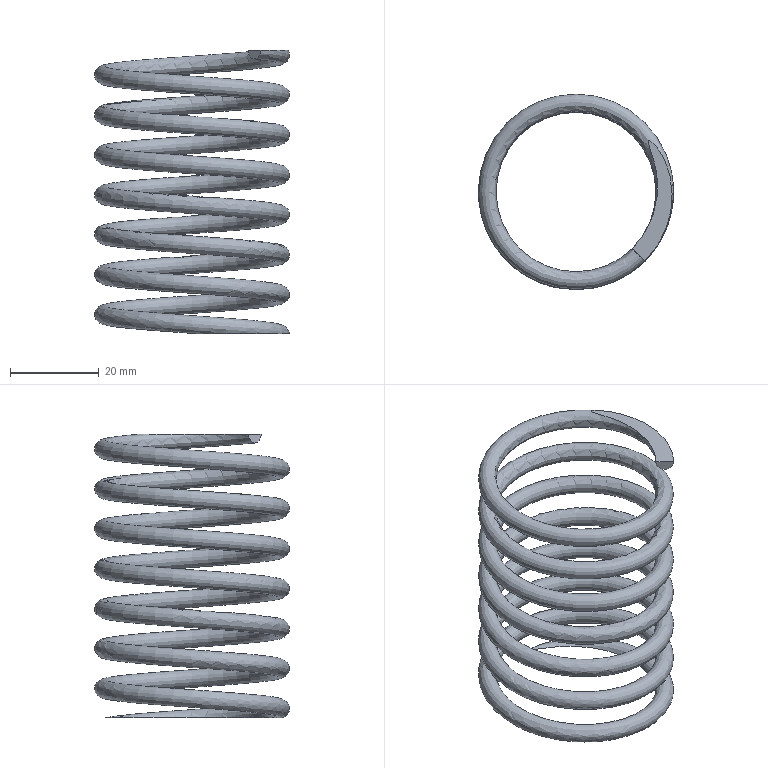Part | NX | features DATUM_CSYS 2, SKETCH 2, DATUM_ON_PATH 1, EXTRUDE 1, HELIX 1, LINE 1, SKIN 1 | 1 solid | 4 faces | box 43.994 x 43.994 x 64 mm | volume 11223 mm3 | plane 3 | spline 1